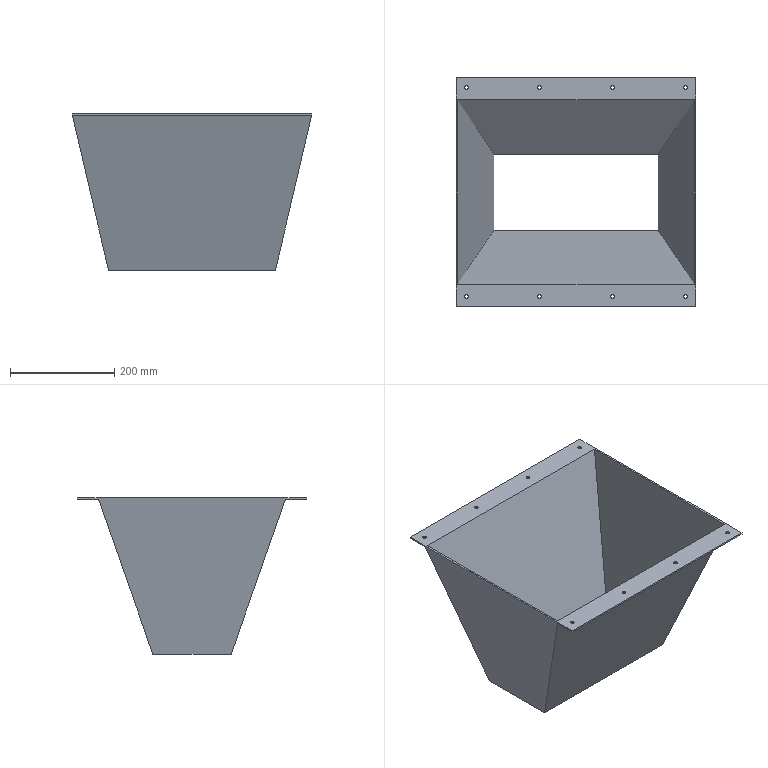Part | SolidWorks | features ICE 7, Extrusion 1, HoleWzd 1, LPattern 1, MirrorPattern 1, Shell 1 | 1 solid | 42 faces | box 460 x 440 x 300 mm | volume 1312965 mm3 | plane 26 | cylinder 16 | commonest cylinder face diameters 7 x16
STEP:
#1=CARTESIAN_POINT('',(206.5,-200.,-3.));
#2=VERTEX_POINT('',#1);
#3=CARTESIAN_POINT('',(213.5,-200.,-3.));
#4=VERTEX_POINT('',#3);
#5=CARTESIAN_POINT('',(210.,-200.,-3.));
#6=DIRECTION('',(0.,0.,1.));
#7=DIRECTION('',(1.,0.,0.));
#8=AXIS2_PLACEMENT_3D('',#5,#6,#7);
#9=CIRCLE('',#8,3.5);
#10=EDGE_CURVE('',#2,#4,#9,.T.);
#11=ORIENTED_EDGE('',*,*,#10,.F.);
#12=CARTESIAN_POINT('',(206.5,-200.,0.));
#13=VERTEX_POINT('',#12);
#14=CARTESIAN_POINT('',(206.5,-200.,0.));
#15=DIRECTION('',(0.,0.,1.));
#16=VECTOR('',#15,1000.);
#17=LINE('',#14,#16);
#18=EDGE_CURVE('',#2,#13,#17,.T.);
#19=ORIENTED_EDGE('',*,*,#18,.T.);
#20=CARTESIAN_POINT('',(213.5,-200.,0.));
#21=VERTEX_POINT('',#20);
#22=CARTESIAN_POINT('',(210.,-200.,0.));
#23=DIRECTION('',(0.,0.,1.));
#24=DIRECTION('',(1.,0.,0.));
#25=AXIS2_PLACEMENT_3D('',#22,#23,#24);
#26=CIRCLE('',#25,3.5);
#27=EDGE_CURVE('',#13,#21,#26,.T.);
#28=ORIENTED_EDGE('',*,*,#27,.T.);
#29=CARTESIAN_POINT('',(213.5,-200.,0.));
#30=DIRECTION('',(0.,0.,1.));
#31=VECTOR('',#30,1000.);
#32=LINE('',#29,#31);
#33=EDGE_CURVE('',#4,#21,#32,.T.);
#34=ORIENTED_EDGE('',*,*,#33,.F.);
#35=EDGE_LOOP('',(#11,#19,#28,#34));
#36=FACE_OUTER_BOUND('',#35,.T.);
#37=CARTESIAN_POINT('',(210.,-200.,0.));
#38=DIRECTION('',(0.,0.,1.));
#39=DIRECTION('',(1.,0.,0.));
#40=AXIS2_PLACEMENT_3D('',#37,#38,#39);
#41=CYLINDRICAL_SURFACE('',#40,3.5);
#42=ADVANCED_FACE('',(#36),#41,.F.);
#43=CARTESIAN_POINT('',(66.5,-200.,-3.));
#44=VERTEX_POINT('',#43);
#45=CARTESIAN_POINT('',(73.5,-200.,-3.));
#46=VERTEX_POINT('',#45);
#47=CARTESIAN_POINT('',(70.,-200.,-3.));
#48=DIRECTION('',(0.,0.,1.));
#49=DIRECTION('',(1.,0.,0.));
#50=AXIS2_PLACEMENT_3D('',#47,#48,#49);
#51=CIRCLE('',#50,3.5);
#52=EDGE_CURVE('',#44,#46,#51,.T.);
#53=ORIENTED_EDGE('',*,*,#52,.F.);
#54=CARTESIAN_POINT('',(66.5,-200.,0.));
#55=VERTEX_POINT('',#54);
#56=CARTESIAN_POINT('',(66.5,-200.,0.));
#57=DIRECTION('',(0.,0.,1.));
#58=VECTOR('',#57,1000.);
#59=LINE('',#56,#58);
#60=EDGE_CURVE('',#44,#55,#59,.T.);
#61=ORIENTED_EDGE('',*,*,#60,.T.);
#62=CARTESIAN_POINT('',(73.5,-200.,0.));
#63=VERTEX_POINT('',#62);
#64=CARTESIAN_POINT('',(70.,-200.,0.));
#65=DIRECTION('',(0.,0.,1.));
#66=DIRECTION('',(1.,0.,0.));
#67=AXIS2_PLACEMENT_3D('',#64,#65,#66);
#68=CIRCLE('',#67,3.5);
#69=EDGE_CURVE('',#55,#63,#68,.T.);
#70=ORIENTED_EDGE('',*,*,#69,.T.);
#71=CARTESIAN_POINT('',(73.5,-200.,0.));
#72=DIRECTION('',(0.,0.,1.));
#73=VECTOR('',#72,1000.);
#74=LINE('',#71,#73);
#75=EDGE_CURVE('',#46,#63,#74,.T.);
#76=ORIENTED_EDGE('',*,*,#75,.F.);
#77=EDGE_LOOP('',(#53,#61,#70,#76));
#78=FACE_OUTER_BOUND('',#77,.T.);
#79=CARTESIAN_POINT('',(70.,-200.,0.));
#80=DIRECTION('',(0.,0.,1.));
#81=DIRECTION('',(1.,0.,0.));
#82=AXIS2_PLACEMENT_3D('',#79,#80,#81);
#83=CYLINDRICAL_SURFACE('',#82,3.5);
#84=ADVANCED_FACE('',(#78),#83,.F.);
#85=CARTESIAN_POINT('',(-73.5,-200.,-3.));
#86=VERTEX_POINT('',#85);
#87=CARTESIAN_POINT('',(-66.5,-200.,-3.));
#88=VERTEX_POINT('',#87);
#89=CARTESIAN_POINT('',(-70.,-200.,-3.));
#90=DIRECTION('',(0.,0.,1.));
#91=DIRECTION('',(1.,0.,0.));
#92=AXIS2_PLACEMENT_3D('',#89,#90,#91);
#93=CIRCLE('',#92,3.5);
#94=EDGE_CURVE('',#86,#88,#93,.T.);
#95=ORIENTED_EDGE('',*,*,#94,.F.);
#96=CARTESIAN_POINT('',(-73.5,-200.,0.));
#97=VERTEX_POINT('',#96);
#98=CARTESIAN_POINT('',(-73.5,-200.,0.));
#99=DIRECTION('',(0.,0.,1.));
#100=VECTOR('',#99,1000.);
#101=LINE('',#98,#100);
#102=EDGE_CURVE('',#86,#97,#101,.T.);
#103=ORIENTED_EDGE('',*,*,#102,.T.);
#104=CARTESIAN_POINT('',(-66.5,-200.,0.));
#105=VERTEX_POINT('',#104);
#106=CARTESIAN_POINT('',(-70.,-200.,0.));
#107=DIRECTION('',(0.,0.,1.));
#108=DIRECTION('',(1.,0.,0.));
#109=AXIS2_PLACEMENT_3D('',#106,#107,#108);
#110=CIRCLE('',#109,3.5);
#111=EDGE_CURVE('',#97,#105,#110,.T.);
#112=ORIENTED_EDGE('',*,*,#111,.T.);
#113=CARTESIAN_POINT('',(-66.5,-200.,0.));
#114=DIRECTION('',(0.,0.,1.));
#115=VECTOR('',#114,1000.);
#116=LINE('',#113,#115);
#117=EDGE_CURVE('',#88,#105,#116,.T.);
#118=ORIENTED_EDGE('',*,*,#117,.F.);
#119=EDGE_LOOP('',(#95,#103,#112,#118));
#120=FACE_OUTER_BOUND('',#119,.T.);
#121=CARTESIAN_POINT('',(-70.,-200.,0.));
#122=DIRECTION('',(0.,0.,1.));
#123=DIRECTION('',(1.,0.,0.));
#124=AXIS2_PLACEMENT_3D('',#121,#122,#123);
#125=CYLINDRICAL_SURFACE('',#124,3.5);
#126=ADVANCED_FACE('',(#120),#125,.F.);
#127=CARTESIAN_POINT('',(-213.5,-200.,-3.));
#128=VERTEX_POINT('',#127);
#129=CARTESIAN_POINT('',(-206.5,-200.,-3.));
#130=VERTEX_POINT('',#129);
#131=CARTESIAN_POINT('',(-210.,-200.,-3.));
#132=DIRECTION('',(0.,0.,1.));
#133=DIRECTION('',(1.,0.,0.));
#134=AXIS2_PLACEMENT_3D('',#131,#132,#133);
#135=CIRCLE('',#134,3.5);
#136=EDGE_CURVE('',#128,#130,#135,.T.);
#137=ORIENTED_EDGE('',*,*,#136,.F.);
#138=CARTESIAN_POINT('',(-213.5,-200.,0.));
#139=VERTEX_POINT('',#138);
#140=CARTESIAN_POINT('',(-213.5,-200.,0.));
#141=DIRECTION('',(0.,0.,1.));
#142=VECTOR('',#141,1000.);
#143=LINE('',#140,#142);
#144=EDGE_CURVE('',#128,#139,#143,.T.);
#145=ORIENTED_EDGE('',*,*,#144,.T.);
#146=CARTESIAN_POINT('',(-206.5,-200.,0.));
#147=VERTEX_POINT('',#146);
#148=CARTESIAN_POINT('',(-210.,-200.,0.));
#149=DIRECTION('',(0.,0.,1.));
#150=DIRECTION('',(1.,0.,0.));
#151=AXIS2_PLACEMENT_3D('',#148,#149,#150);
#152=CIRCLE('',#151,3.5);
#153=EDGE_CURVE('',#139,#147,#152,.T.);
#154=ORIENTED_EDGE('',*,*,#153,.T.);
#155=CARTESIAN_POINT('',(-206.5,-200.,0.));
#156=DIRECTION('',(0.,0.,1.));
#157=VECTOR('',#156,1000.);
#158=LINE('',#155,#157);
#159=EDGE_CURVE('',#130,#147,#158,.T.);
#160=ORIENTED_EDGE('',*,*,#159,.F.);
#161=EDGE_LOOP('',(#137,#145,#154,#160));
#162=FACE_OUTER_BOUND('',#161,.T.);
#163=CARTESIAN_POINT('',(-210.,-200.,0.));
#164=DIRECTION('',(0.,0.,1.));
#165=DIRECTION('',(1.,0.,0.));
#166=AXIS2_PLACEMENT_3D('',#163,#164,#165);
#167=CYLINDRICAL_SURFACE('',#166,3.5);
#168=ADVANCED_FACE('',(#162),#167,.F.);
#169=CARTESIAN_POINT('',(206.5,200.,-3.));
#170=VERTEX_POINT('',#169);
#171=CARTESIAN_POINT('',(213.5,200.,-3.));
#172=VERTEX_POINT('',#171);
#173=CARTESIAN_POINT('',(210.,200.,-3.));
#174=DIRECTION('',(0.,0.,1.));
#175=DIRECTION('',(1.,0.,0.));
#176=AXIS2_PLACEMENT_3D('',#173,#174,#175);
#177=CIRCLE('',#176,3.5);
#178=EDGE_CURVE('',#170,#172,#177,.T.);
#179=ORIENTED_EDGE('',*,*,#178,.F.);
#180=CARTESIAN_POINT('',(206.5,200.,0.));
#181=VERTEX_POINT('',#180);
#182=CARTESIAN_POINT('',(206.5,200.,0.));
#183=DIRECTION('',(0.,0.,1.));
#184=VECTOR('',#183,1000.);
#185=LINE('',#182,#184);
#186=EDGE_CURVE('',#170,#181,#185,.T.);
#187=ORIENTED_EDGE('',*,*,#186,.T.);
#188=CARTESIAN_POINT('',(213.5,200.,0.));
#189=VERTEX_POINT('',#188);
#190=CARTESIAN_POINT('',(210.,200.,0.));
#191=DIRECTION('',(0.,0.,1.));
#192=DIRECTION('',(1.,0.,0.));
#193=AXIS2_PLACEMENT_3D('',#190,#191,#192);
#194=CIRCLE('',#193,3.5);
#195=EDGE_CURVE('',#181,#189,#194,.T.);
#196=ORIENTED_EDGE('',*,*,#195,.T.);
#197=CARTESIAN_POINT('',(213.5,200.,0.));
#198=DIRECTION('',(0.,0.,1.));
#199=VECTOR('',#198,1000.);
#200=LINE('',#197,#199);
#201=EDGE_CURVE('',#172,#189,#200,.T.);
#202=ORIENTED_EDGE('',*,*,#201,.F.);
#203=EDGE_LOOP('',(#179,#187,#196,#202));
#204=FACE_OUTER_BOUND('',#203,.T.);
#205=CARTESIAN_POINT('',(210.,200.,0.));
#206=DIRECTION('',(0.,0.,1.));
#207=DIRECTION('',(1.,0.,0.));
#208=AXIS2_PLACEMENT_3D('',#205,#206,#207);
#209=CYLINDRICAL_SURFACE('',#208,3.5);
#210=ADVANCED_FACE('',(#204),#209,.F.);
#211=CARTESIAN_POINT('',(66.5,200.,-3.));
#212=VERTEX_POINT('',#211);
#213=CARTESIAN_POINT('',(73.5,200.,-3.));
#214=VERTEX_POINT('',#213);
#215=CARTESIAN_POINT('',(70.,200.,-3.));
#216=DIRECTION('',(0.,0.,1.));
#217=DIRECTION('',(1.,0.,0.));
#218=AXIS2_PLACEMENT_3D('',#215,#216,#217);
#219=CIRCLE('',#218,3.5);
#220=EDGE_CURVE('',#212,#214,#219,.T.);
#221=ORIENTED_EDGE('',*,*,#220,.F.);
#222=CARTESIAN_POINT('',(66.5,200.,0.));
#223=VERTEX_POINT('',#222);
#224=CARTESIAN_POINT('',(66.5,200.,0.));
#225=DIRECTION('',(0.,0.,1.));
#226=VECTOR('',#225,1000.);
#227=LINE('',#224,#226);
#228=EDGE_CURVE('',#212,#223,#227,.T.);
#229=ORIENTED_EDGE('',*,*,#228,.T.);
#230=CARTESIAN_POINT('',(73.5,200.,0.));
#231=VERTEX_POINT('',#230);
#232=CARTESIAN_POINT('',(70.,200.,0.));
#233=DIRECTION('',(0.,0.,1.));
#234=DIRECTION('',(1.,0.,0.));
#235=AXIS2_PLACEMENT_3D('',#232,#233,#234);
#236=CIRCLE('',#235,3.5);
#237=EDGE_CURVE('',#223,#231,#236,.T.);
#238=ORIENTED_EDGE('',*,*,#237,.T.);
#239=CARTESIAN_POINT('',(73.5,200.,0.));
#240=DIRECTION('',(0.,0.,1.));
#241=VECTOR('',#240,1000.);
#242=LINE('',#239,#241);
#243=EDGE_CURVE('',#214,#231,#242,.T.);
#244=ORIENTED_EDGE('',*,*,#243,.F.);
#245=EDGE_LOOP('',(#221,#229,#238,#244));
#246=FACE_OUTER_BOUND('',#245,.T.);
#247=CARTESIAN_POINT('',(70.,200.,0.));
#248=DIRECTION('',(0.,0.,1.));
#249=DIRECTION('',(1.,0.,0.));
#250=AXIS2_PLACEMENT_3D('',#247,#248,#249);
#251=CYLINDRICAL_SURFACE('',#250,3.5);
#252=ADVANCED_FACE('',(#246),#251,.F.);
#253=CARTESIAN_POINT('',(-73.5,200.,-3.));
#254=VERTEX_POINT('',#253);
#255=CARTESIAN_POINT('',(-66.5,200.,-3.));
#256=VERTEX_POINT('',#255);
#257=CARTESIAN_POINT('',(-70.,200.,-3.));
#258=DIRECTION('',(0.,0.,1.));
#259=DIRECTION('',(1.,0.,0.));
#260=AXIS2_PLACEMENT_3D('',#257,#258,#259);
#261=CIRCLE('',#260,3.5);
#262=EDGE_CURVE('',#254,#256,#261,.T.);
#263=ORIENTED_EDGE('',*,*,#262,.F.);
#264=CARTESIAN_POINT('',(-73.5,200.,0.));
#265=VERTEX_POINT('',#264);
#266=CARTESIAN_POINT('',(-73.5,200.,0.));
#267=DIRECTION('',(0.,0.,1.));
#268=VECTOR('',#267,1000.);
#269=LINE('',#266,#268);
#270=EDGE_CURVE('',#254,#265,#269,.T.);
#271=ORIENTED_EDGE('',*,*,#270,.T.);
#272=CARTESIAN_POINT('',(-66.5,200.,0.));
#273=VERTEX_POINT('',#272);
#274=CARTESIAN_POINT('',(-70.,200.,0.));
#275=DIRECTION('',(0.,0.,1.));
#276=DIRECTION('',(1.,0.,0.));
#277=AXIS2_PLACEMENT_3D('',#274,#275,#276);
#278=CIRCLE('',#277,3.5);
#279=EDGE_CURVE('',#265,#273,#278,.T.);
#280=ORIENTED_EDGE('',*,*,#279,.T.);
#281=CARTESIAN_POINT('',(-66.5,200.,0.));
#282=DIRECTION('',(0.,0.,1.));
#283=VECTOR('',#282,1000.);
#284=LINE('',#281,#283);
#285=EDGE_CURVE('',#256,#273,#284,.T.);
#286=ORIENTED_EDGE('',*,*,#285,.F.);
#287=EDGE_LOOP('',(#263,#271,#280,#286));
#288=FACE_OUTER_BOUND('',#287,.T.);
#289=CARTESIAN_POINT('',(-70.,200.,0.));
#290=DIRECTION('',(0.,0.,1.));
#291=DIRECTION('',(1.,0.,0.));
#292=AXIS2_PLACEMENT_3D('',#289,#290,#291);
#293=CYLINDRICAL_SURFACE('',#292,3.5);
#294=ADVANCED_FACE('',(#288),#293,.F.);
#295=CARTESIAN_POINT('',(-213.5,200.,-3.));
#296=VERTEX_POINT('',#295);
#297=CARTESIAN_POINT('',(-206.5,200.,-3.));
#298=VERTEX_POINT('',#297);
#299=CARTESIAN_POINT('',(-210.,200.,-3.));
#300=DIRECTION('',(0.,0.,1.));
#301=DIRECTION('',(1.,0.,0.));
#302=AXIS2_PLACEMENT_3D('',#299,#300,#301);
#303=CIRCLE('',#302,3.5);
#304=EDGE_CURVE('',#296,#298,#303,.T.);
#305=ORIENTED_EDGE('',*,*,#304,.F.);
#306=CARTESIAN_POINT('',(-213.5,200.,0.));
#307=VERTEX_POINT('',#306);
#308=CARTESIAN_POINT('',(-213.5,200.,0.));
#309=DIRECTION('',(0.,0.,1.));
#310=VECTOR('',#309,1000.);
#311=LINE('',#308,#310);
#312=EDGE_CURVE('',#296,#307,#311,.T.);
#313=ORIENTED_EDGE('',*,*,#312,.T.);
#314=CARTESIAN_POINT('',(-206.5,200.,0.));
#315=VERTEX_POINT('',#314);
#316=CARTESIAN_POINT('',(-210.,200.,0.));
#317=DIRECTION('',(0.,0.,1.));
#318=DIRECTION('',(1.,0.,0.));
#319=AXIS2_PLACEMENT_3D('',#316,#317,#318);
#320=CIRCLE('',#319,3.5);
#321=EDGE_CURVE('',#307,#315,#320,.T.);
#322=ORIENTED_EDGE('',*,*,#321,.T.);
#323=CARTESIAN_POINT('',(-206.5,200.,0.));
#324=DIRECTION('',(0.,0.,1.));
#325=VECTOR('',#324,1000.);
#326=LINE('',#323,#325);
#327=EDGE_CURVE('',#298,#315,#326,.T.);
#328=ORIENTED_EDGE('',*,*,#327,.F.);
#329=EDGE_LOOP('',(#305,#313,#322,#328));
#330=FACE_OUTER_BOUND('',#329,.T.);
#331=CARTESIAN_POINT('',(-210.,200.,0.));
#332=DIRECTION('',(0.,0.,1.));
#333=DIRECTION('',(1.,0.,0.));
#334=AXIS2_PLACEMENT_3D('',#331,#332,#333);
#335=CYLINDRICAL_SURFACE('',#334,3.5);
#336=ADVANCED_FACE('',(#330),#335,.F.);
#337=CARTESIAN_POINT('',(-157.619,-72.872,-300.));
#338=VERTEX_POINT('',#337);
#339=CARTESIAN_POINT('',(157.619,-72.872,-300.));
#340=VERTEX_POINT('',#339);
#341=CARTESIAN_POINT('',(-157.619,-72.872,-300.));
#342=DIRECTION('',(1.,0.,0.));
#343=VECTOR('',#342,1000.);
#344=LINE('',#341,#343);
#345=EDGE_CURVE('',#338,#340,#344,.T.);
#346=ORIENTED_EDGE('',*,*,#345,.T.);
#347=CARTESIAN_POINT('',(157.619,72.872,-300.));
#348=VERTEX_POINT('',#347);
#349=CARTESIAN_POINT('',(157.619,-72.872,-300.));
#350=DIRECTION('',(0.,1.,0.));
#351=VECTOR('',#350,1000.);
#352=LINE('',#349,#351);
#353=EDGE_CURVE('',#340,#348,#352,.T.);
#354=ORIENTED_EDGE('',*,*,#353,.T.);
#355=CARTESIAN_POINT('',(-157.619,72.872,-300.));
#356=VERTEX_POINT('',#355);
#357=CARTESIAN_POINT('',(157.619,72.872,-300.));
#358=DIRECTION('',(-1.,0.,0.));
#359=VECTOR('',#358,1000.);
#360=LINE('',#357,#359);
#361=EDGE_CURVE('',#348,#356,#360,.T.);
#362=ORIENTED_EDGE('',*,*,#361,.T.);
#363=CARTESIAN_POINT('',(-157.619,72.872,-300.));
#364=DIRECTION('',(0.,-1.,0.));
#365=VECTOR('',#364,1000.);
#366=LINE('',#363,#365);
#367=EDGE_CURVE('',#356,#338,#366,.T.);
#368=ORIENTED_EDGE('',*,*,#367,.T.);
#369=EDGE_LOOP('',(#346,#354,#362,#368));
#370=FACE_BOUND('',#369,.T.);
#371=CARTESIAN_POINT('',(-160.,75.,-300.));
#372=VERTEX_POINT('',#371);
#373=CARTESIAN_POINT('',(160.,75.,-300.));
#374=VERTEX_POINT('',#373);
#375=CARTESIAN_POINT('',(-230.,75.,-300.));
#376=DIRECTION('',(1.,0.,0.));
#377=VECTOR('',#376,1000.);
#378=LINE('',#375,#377);
#379=EDGE_CURVE('',#372,#374,#378,.T.);
#380=ORIENTED_EDGE('',*,*,#379,.T.);
#381=CARTESIAN_POINT('',(160.,-75.,-300.));
#382=VERTEX_POINT('',#381);
#383=CARTESIAN_POINT('',(160.,-302.,-300.));
#384=DIRECTION('',(0.,1.,0.));
#385=VECTOR('',#384,1000.);
#386=LINE('',#383,#385);
#387=EDGE_CURVE('',#382,#374,#386,.T.);
#388=ORIENTED_EDGE('',*,*,#387,.F.);
#389=CARTESIAN_POINT('',(-160.,-75.,-300.));
#390=VERTEX_POINT('',#389);
#391=CARTESIAN_POINT('',(-230.,-75.,-300.));
#392=DIRECTION('',(1.,0.,0.));
#393=VECTOR('',#392,1000.);
#394=LINE('',#391,#393);
#395=EDGE_CURVE('',#390,#382,#394,.T.);
#396=ORIENTED_EDGE('',*,*,#395,.F.);
#397=CARTESIAN_POINT('',(-160.,-302.,-300.));
#398=DIRECTION('',(0.,1.,0.));
#399=VECTOR('',#398,1000.);
#400=LINE('',#397,#399);
#401=EDGE_CURVE('',#390,#372,#400,.T.);
#402=ORIENTED_EDGE('',*,*,#401,.T.);
#403=EDGE_LOOP('',(#380,#388,#396,#402));
#404=FACE_OUTER_BOUND('',#403,.T.);
#405=CARTESIAN_POINT('',(0.,0.,-300.));
#406=DIRECTION('',(0.,0.,1.));
#407=DIRECTION('',(1.,0.,0.));
#408=AXIS2_PLACEMENT_3D('',#405,#406,#407);
#409=PLANE('',#408);
#410=ADVANCED_FACE('',(#370,#404),#409,.F.);
#411=CARTESIAN_POINT('',(210.,-200.,0.));
#412=DIRECTION('',(0.,0.,1.));
#413=DIRECTION('',(1.,0.,0.));
#414=AXIS2_PLACEMENT_3D('',#411,#412,#413);
#415=CIRCLE('',#414,3.5);
#416=EDGE_CURVE('',#21,#13,#415,.T.);
#417=ORIENTED_EDGE('',*,*,#416,.F.);
#418=ORIENTED_EDGE('',*,*,#27,.F.);
#419=EDGE_LOOP('',(#417,#418));
#420=FACE_BOUND('',#419,.T.);
#421=CARTESIAN_POINT('',(70.,-200.,0.));
#422=DIRECTION('',(0.,0.,1.));
#423=DIRECTION('',(1.,0.,0.));
#424=AXIS2_PLACEMENT_3D('',#421,#422,#423);
#425=CIRCLE('',#424,3.5);
#426=EDGE_CURVE('',#63,#55,#425,.T.);
#427=ORIENTED_EDGE('',*,*,#426,.F.);
#428=ORIENTED_EDGE('',*,*,#69,.F.);
#429=EDGE_LOOP('',(#427,#428));
#430=FACE_BOUND('',#429,.T.);
#431=CARTESIAN_POINT('',(-70.,-200.,0.));
#432=DIRECTION('',(0.,0.,1.));
#433=DIRECTION('',(1.,0.,0.));
#434=AXIS2_PLACEMENT_3D('',#431,#432,#433);
#435=CIRCLE('',#434,3.5);
#436=EDGE_CURVE('',#105,#97,#435,.T.);
#437=ORIENTED_EDGE('',*,*,#436,.F.);
#438=ORIENTED_EDGE('',*,*,#111,.F.);
#439=EDGE_LOOP('',(#437,#438));
#440=FACE_BOUND('',#439,.T.);
#441=CARTESIAN_POINT('',(-210.,-200.,0.));
#442=DIRECTION('',(0.,0.,1.));
#443=DIRECTION('',(1.,0.,0.));
#444=AXIS2_PLACEMENT_3D('',#441,#442,#443);
#445=CIRCLE('',#444,3.5);
#446=EDGE_CURVE('',#147,#139,#445,.T.);
#447=ORIENTED_EDGE('',*,*,#446,.F.);
#448=ORIENTED_EDGE('',*,*,#153,.F.);
#449=EDGE_LOOP('',(#447,#448));
#450=FACE_BOUND('',#449,.T.);
#451=CARTESIAN_POINT('',(-70.,200.,0.));
#452=DIRECTION('',(0.,0.,1.));
#453=DIRECTION('',(1.,0.,0.));
#454=AXIS2_PLACEMENT_3D('',#451,#452,#453);
#455=CIRCLE('',#454,3.5);
#456=EDGE_CURVE('',#273,#265,#455,.T.);
#457=ORIENTED_EDGE('',*,*,#456,.F.);
#458=ORIENTED_EDGE('',*,*,#279,.F.);
#459=EDGE_LOOP('',(#457,#458));
#460=FACE_BOUND('',#459,.T.);
#461=CARTESIAN_POINT('',(-210.,200.,0.));
#462=DIRECTION('',(0.,0.,1.));
#463=DIRECTION('',(1.,0.,0.));
#464=AXIS2_PLACEMENT_3D('',#461,#462,#463);
#465=CIRCLE('',#464,3.5);
#466=EDGE_CURVE('',#315,#307,#465,.T.);
#467=ORIENTED_EDGE('',*,*,#466,.F.);
#468=ORIENTED_EDGE('',*,*,#321,.F.);
#469=EDGE_LOOP('',(#467,#468));
#470=FACE_BOUND('',#469,.T.);
#471=CARTESIAN_POINT('',(226.919,-176.822,0.));
#472=VERTEX_POINT('',#471);
#473=CARTESIAN_POINT('',(226.919,176.822,0.));
#474=VERTEX_POINT('',#473);
#475=CARTESIAN_POINT('',(226.919,-302.,0.));
#476=DIRECTION('',(0.,1.,0.));
#477=VECTOR('',#476,1000.);
#478=LINE('',#475,#477);
#479=EDGE_CURVE('',#472,#474,#478,.T.);
#480=ORIENTED_EDGE('',*,*,#479,.F.);
#481=CARTESIAN_POINT('',(-226.919,-176.822,0.));
#482=VERTEX_POINT('',#481);
#483=CARTESIAN_POINT('',(-230.,-176.822,0.));
#484=DIRECTION('',(1.,0.,0.));
#485=VECTOR('',#484,1000.);
#486=LINE('',#483,#485);
#487=EDGE_CURVE('',#482,#472,#486,.T.);
#488=ORIENTED_EDGE('',*,*,#487,.F.);
#489=CARTESIAN_POINT('',(-226.919,176.822,0.));
#490=VERTEX_POINT('',#489);
#491=CARTESIAN_POINT('',(-226.919,-302.,0.));
#492=DIRECTION('',(0.,-1.,0.));
#493=VECTOR('',#492,1000.);
#494=LINE('',#491,#493);
#495=EDGE_CURVE('',#490,#482,#494,.T.);
#496=ORIENTED_EDGE('',*,*,#495,.F.);
#497=CARTESIAN_POINT('',(-230.,176.822,0.));
#498=DIRECTION('',(-1.,0.,0.));
#499=VECTOR('',#498,1000.);
#500=LINE('',#497,#499);
#501=EDGE_CURVE('',#474,#490,#500,.T.);
#502=ORIENTED_EDGE('',*,*,#501,.F.);
#503=EDGE_LOOP('',(#480,#488,#496,#502));
#504=FACE_BOUND('',#503,.T.);
#505=CARTESIAN_POINT('',(230.,-180.,0.));
#506=VERTEX_POINT('',#505);
#507=CARTESIAN_POINT('',(230.,180.,0.));
#508=VERTEX_POINT('',#507);
#509=CARTESIAN_POINT('',(230.,180.,0.));
#510=DIRECTION('',(0.,1.,0.));
#511=VECTOR('',#510,1000.);
#512=LINE('',#509,#511);
#513=EDGE_CURVE('',#506,#508,#512,.T.);
#514=ORIENTED_EDGE('',*,*,#513,.T.);
#515=CARTESIAN_POINT('',(230.,220.,0.));
#516=VERTEX_POINT('',#515);
#517=CARTESIAN_POINT('',(230.,180.,0.));
#518=DIRECTION('',(0.,1.,0.));
#519=VECTOR('',#518,1000.);
#520=LINE('',#517,#519);
#521=EDGE_CURVE('',#508,#516,#520,.T.);
#522=ORIENTED_EDGE('',*,*,#521,.T.);
#523=CARTESIAN_POINT('',(-230.,220.,0.));
#524=VERTEX_POINT('',#523);
#525=CARTESIAN_POINT('',(-230.,220.,0.));
#526=DIRECTION('',(-1.,0.,0.));
#527=VECTOR('',#526,1000.);
#528=LINE('',#525,#527);
#529=EDGE_CURVE('',#516,#524,#528,.T.);
#530=ORIENTED_EDGE('',*,*,#529,.T.);
#531=CARTESIAN_POINT('',(-230.,180.,0.));
#532=VERTEX_POINT('',#531);
#533=CARTESIAN_POINT('',(-230.,180.,0.));
#534=DIRECTION('',(0.,-1.,0.));
#535=VECTOR('',#534,1000.);
#536=LINE('',#533,#535);
#537=EDGE_CURVE('',#524,#532,#536,.T.);
#538=ORIENTED_EDGE('',*,*,#537,.T.);
#539=CARTESIAN_POINT('',(-230.,-180.,0.));
#540=VERTEX_POINT('',#539);
#541=CARTESIAN_POINT('',(-230.,180.,0.));
#542=DIRECTION('',(0.,-1.,0.));
#543=VECTOR('',#542,1000.);
#544=LINE('',#541,#543);
#545=EDGE_CURVE('',#532,#540,#544,.T.);
#546=ORIENTED_EDGE('',*,*,#545,.T.);
#547=CARTESIAN_POINT('',(-230.,-220.,0.));
#548=VERTEX_POINT('',#547);
#549=CARTESIAN_POINT('',(-230.,-180.,0.));
#550=DIRECTION('',(0.,-1.,0.));
#551=VECTOR('',#550,1000.);
#552=LINE('',#549,#551);
#553=EDGE_CURVE('',#540,#548,#552,.T.);
#554=ORIENTED_EDGE('',*,*,#553,.T.);
#555=CARTESIAN_POINT('',(230.,-220.,0.));
#556=VERTEX_POINT('',#555);
#557=CARTESIAN_POINT('',(-230.,-220.,0.));
#558=DIRECTION('',(1.,0.,0.));
#559=VECTOR('',#558,1000.);
#560=LINE('',#557,#559);
#561=EDGE_CURVE('',#548,#556,#560,.T.);
#562=ORIENTED_EDGE('',*,*,#561,.T.);
#563=CARTESIAN_POINT('',(230.,-180.,0.));
#564=DIRECTION('',(0.,1.,0.));
#565=VECTOR('',#564,1000.);
#566=LINE('',#563,#565);
#567=EDGE_CURVE('',#556,#506,#566,.T.);
#568=ORIENTED_EDGE('',*,*,#567,.T.);
#569=EDGE_LOOP('',(#514,#522,#530,#538,#546,#554,#562,#568));
#570=FACE_OUTER_BOUND('',#569,.T.);
#571=CARTESIAN_POINT('',(70.,200.,0.));
#572=DIRECTION('',(0.,0.,1.));
#573=DIRECTION('',(1.,0.,0.));
#574=AXIS2_PLACEMENT_3D('',#571,#572,#573);
#575=CIRCLE('',#574,3.5);
#576=EDGE_CURVE('',#231,#223,#575,.T.);
#577=ORIENTED_EDGE('',*,*,#576,.F.);
#578=ORIENTED_EDGE('',*,*,#237,.F.);
#579=EDGE_LOOP('',(#577,#578));
#580=FACE_BOUND('',#579,.T.);
#581=CARTESIAN_POINT('',(210.,200.,0.));
#582=DIRECTION('',(0.,0.,1.));
#583=DIRECTION('',(1.,0.,0.));
#584=AXIS2_PLACEMENT_3D('',#581,#582,#583);
#585=CIRCLE('',#584,3.5);
#586=EDGE_CURVE('',#189,#181,#585,.T.);
#587=ORIENTED_EDGE('',*,*,#586,.F.);
#588=ORIENTED_EDGE('',*,*,#195,.F.);
#589=EDGE_LOOP('',(#587,#588));
#590=FACE_BOUND('',#589,.T.);
#591=CARTESIAN_POINT('',(0.,0.,0.));
#592=DIRECTION('',(0.,0.,1.));
#593=DIRECTION('',(1.,0.,0.));
#594=AXIS2_PLACEMENT_3D('',#591,#592,#593);
#595=PLANE('',#594);
#596=ADVANCED_FACE('',(#420,#430,#440,#450,#460,#470,#504,#570,#580,#590),#595,.T.);
#597=CARTESIAN_POINT('',(-229.3,178.95,-3.));
#598=VERTEX_POINT('',#597);
#599=CARTESIAN_POINT('',(-230.,180.,0.));
#600=DIRECTION('',(-0.2151,0.3226,0.9218));
#601=VECTOR('',#600,1000.);
#602=LINE('',#599,#601);
#603=EDGE_CURVE('',#372,#598,#602,.T.);
#604=ORIENTED_EDGE('',*,*,#603,.T.);
#605=CARTESIAN_POINT('',(229.3,178.95,-3.));
#606=VERTEX_POINT('',#605);
#607=CARTESIAN_POINT('',(-230.,178.95,-3.));
#608=DIRECTION('',(1.,0.,0.));
#609=VECTOR('',#608,1000.);
#610=LINE('',#607,#609);
#611=EDGE_CURVE('',#598,#606,#610,.T.);
#612=ORIENTED_EDGE('',*,*,#611,.T.);
#613=CARTESIAN_POINT('',(208.721,148.081,-91.197));
#614=DIRECTION('',(-0.2151,-0.3226,-0.9218));
#615=VECTOR('',#614,1000.);
#616=LINE('',#613,#615);
#617=EDGE_CURVE('',#606,#374,#616,.T.);
#618=ORIENTED_EDGE('',*,*,#617,.T.);
#619=ORIENTED_EDGE('',*,*,#379,.F.);
#620=EDGE_LOOP('',(#604,#612,#618,#619));
#621=FACE_OUTER_BOUND('',#620,.T.);
#622=CARTESIAN_POINT('',(-230.,180.,0.));
#623=DIRECTION('',(0.,-0.9439,0.3304));
#624=DIRECTION('',(0.,-0.3304,-0.9439));
#625=AXIS2_PLACEMENT_3D('',#622,#623,#624);
#626=PLANE('',#625);
#627=ADVANCED_FACE('',(#621),#626,.F.);
#628=CARTESIAN_POINT('',(229.3,-178.95,-3.));
#629=VERTEX_POINT('',#628);
#630=CARTESIAN_POINT('',(208.721,-148.081,-91.197));
#631=DIRECTION('',(0.2151,-0.3226,0.9218));
#632=VECTOR('',#631,1000.);
#633=LINE('',#630,#632);
#634=EDGE_CURVE('',#382,#629,#633,.T.);
#635=ORIENTED_EDGE('',*,*,#634,.T.);
#636=CARTESIAN_POINT('',(-229.3,-178.95,-3.));
#637=VERTEX_POINT('',#636);
#638=CARTESIAN_POINT('',(230.,-178.95,-3.));
#639=DIRECTION('',(-1.,0.,0.));
#640=VECTOR('',#639,1000.);
#641=LINE('',#638,#640);
#642=EDGE_CURVE('',#629,#637,#641,.T.);
#643=ORIENTED_EDGE('',*,*,#642,.T.);
#644=CARTESIAN_POINT('',(-230.,-180.,0.));
#645=DIRECTION('',(0.2151,0.3226,-0.9218));
#646=VECTOR('',#645,1000.);
#647=LINE('',#644,#646);
#648=EDGE_CURVE('',#637,#390,#647,.T.);
#649=ORIENTED_EDGE('',*,*,#648,.T.);
#650=ORIENTED_EDGE('',*,*,#395,.T.);
#651=EDGE_LOOP('',(#635,#643,#649,#650));
#652=FACE_OUTER_BOUND('',#651,.T.);
#653=CARTESIAN_POINT('',(-230.,-180.,0.));
#654=DIRECTION('',(0.,0.9439,0.3304));
#655=DIRECTION('',(0.,-0.3304,0.9439));
#656=AXIS2_PLACEMENT_3D('',#653,#654,#655);
#657=PLANE('',#656);
#658=ADVANCED_FACE('',(#652),#657,.F.);
#659=ORIENTED_EDGE('',*,*,#401,.F.);
#660=ORIENTED_EDGE('',*,*,#648,.F.);
#661=CARTESIAN_POINT('',(-230.,-180.,0.));
#662=DIRECTION('',(0.2151,0.3226,-0.9218));
#663=VECTOR('',#662,1000.);
#664=LINE('',#661,#663);
#665=EDGE_CURVE('',#540,#637,#664,.T.);
#666=ORIENTED_EDGE('',*,*,#665,.F.);
#667=ORIENTED_EDGE('',*,*,#545,.F.);
#668=CARTESIAN_POINT('',(-230.,180.,0.));
#669=DIRECTION('',(-0.2151,0.3226,0.9218));
#670=VECTOR('',#669,1000.);
#671=LINE('',#668,#670);
#672=EDGE_CURVE('',#598,#532,#671,.T.);
#673=ORIENTED_EDGE('',*,*,#672,.F.);
#674=ORIENTED_EDGE('',*,*,#603,.F.);
#675=EDGE_LOOP('',(#659,#660,#666,#667,#673,#674));
#676=FACE_OUTER_BOUND('',#675,.T.);
#677=CARTESIAN_POINT('',(-230.,-302.,0.));
#678=DIRECTION('',(0.9738,0.,0.2272));
#679=DIRECTION('',(0.2272,0.,-0.9738));
#680=AXIS2_PLACEMENT_3D('',#677,#678,#679);
#681=PLANE('',#680);
#682=ADVANCED_FACE('',(#676),#681,.F.);
#683=ORIENTED_EDGE('',*,*,#513,.F.);
#684=CARTESIAN_POINT('',(208.721,-148.081,-91.197));
#685=DIRECTION('',(0.2151,-0.3226,0.9218));
#686=VECTOR('',#685,1000.);
#687=LINE('',#684,#686);
#688=EDGE_CURVE('',#629,#506,#687,.T.);
#689=ORIENTED_EDGE('',*,*,#688,.F.);
#690=ORIENTED_EDGE('',*,*,#634,.F.);
#691=ORIENTED_EDGE('',*,*,#387,.T.);
#692=ORIENTED_EDGE('',*,*,#617,.F.);
#693=CARTESIAN_POINT('',(208.721,148.081,-91.197));
#694=DIRECTION('',(-0.2151,-0.3226,-0.9218));
#695=VECTOR('',#694,1000.);
#696=LINE('',#693,#695);
#697=EDGE_CURVE('',#508,#606,#696,.T.);
#698=ORIENTED_EDGE('',*,*,#697,.F.);
#699=EDGE_LOOP('',(#683,#689,#690,#691,#692,#698));
#700=FACE_OUTER_BOUND('',#699,.T.);
#701=CARTESIAN_POINT('',(230.,-302.,0.));
#702=DIRECTION('',(-0.9738,0.,0.2272));
#703=DIRECTION('',(0.2272,0.,0.9738));
#704=AXIS2_PLACEMENT_3D('',#701,#702,#703);
#705=PLANE('',#704);
#706=ADVANCED_FACE('',(#700),#705,.F.);
#707=ORIENTED_EDGE('',*,*,#501,.T.);
#708=CARTESIAN_POINT('',(-157.619,72.872,-297.));
#709=VERTEX_POINT('',#708);
#710=CARTESIAN_POINT('',(-227.282,177.366,1.556));
#711=DIRECTION('',(-0.2151,0.3226,0.9218));
#712=VECTOR('',#711,1000.);
#713=LINE('',#710,#712);
#714=EDGE_CURVE('',#709,#490,#713,.T.);
#715=ORIENTED_EDGE('',*,*,#714,.F.);
#716=CARTESIAN_POINT('',(157.619,72.872,-297.));
#717=VERTEX_POINT('',#716);
#718=CARTESIAN_POINT('',(0.,72.872,-297.));
#719=DIRECTION('',(1.,0.,0.));
#720=VECTOR('',#719,1000.);
#721=LINE('',#718,#720);
#722=EDGE_CURVE('',#709,#717,#721,.T.);
#723=ORIENTED_EDGE('',*,*,#722,.T.);
#724=CARTESIAN_POINT('',(206.003,145.447,-89.641));
#725=DIRECTION('',(-0.2151,-0.3226,-0.9218));
#726=VECTOR('',#725,1000.);
#727=LINE('',#724,#726);
#728=EDGE_CURVE('',#474,#717,#727,.T.);
#729=ORIENTED_EDGE('',*,*,#728,.F.);
#730=EDGE_LOOP('',(#707,#715,#723,#729));
#731=FACE_OUTER_BOUND('',#730,.T.);
#732=CARTESIAN_POINT('',(-230.,177.168,0.9911));
#733=DIRECTION('',(0.,-0.9439,0.3304));
#734=DIRECTION('',(0.,-0.3304,-0.9439));
#735=AXIS2_PLACEMENT_3D('',#732,#733,#734);
#736=PLANE('',#735);
#737=ADVANCED_FACE('',(#731),#736,.T.);
#738=CARTESIAN_POINT('',(-157.619,-72.872,-297.));
#739=VERTEX_POINT('',#738);
#740=CARTESIAN_POINT('',(157.619,-72.872,-297.));
#741=VERTEX_POINT('',#740);
#742=CARTESIAN_POINT('',(-230.,-72.872,-297.));
#743=DIRECTION('',(1.,0.,0.));
#744=VECTOR('',#743,1000.);
#745=LINE('',#742,#744);
#746=EDGE_CURVE('',#739,#741,#745,.T.);
#747=ORIENTED_EDGE('',*,*,#746,.F.);
#748=CARTESIAN_POINT('',(-227.282,-177.366,1.556));
#749=DIRECTION('',(0.2151,0.3226,-0.9218));
#750=VECTOR('',#749,1000.);
#751=LINE('',#748,#750);
#752=EDGE_CURVE('',#482,#739,#751,.T.);
#753=ORIENTED_EDGE('',*,*,#752,.F.);
#754=ORIENTED_EDGE('',*,*,#487,.T.);
#755=CARTESIAN_POINT('',(206.003,-145.447,-89.641));
#756=DIRECTION('',(0.2151,-0.3226,0.9218));
#757=VECTOR('',#756,1000.);
#758=LINE('',#755,#757);
#759=EDGE_CURVE('',#741,#472,#758,.T.);
#760=ORIENTED_EDGE('',*,*,#759,.F.);
#761=EDGE_LOOP('',(#747,#753,#754,#760));
#762=FACE_OUTER_BOUND('',#761,.T.);
#763=CARTESIAN_POINT('',(-230.,-177.168,0.9911));
#764=DIRECTION('',(0.,0.9439,0.3304));
#765=DIRECTION('',(0.,-0.3304,0.9439));
#766=AXIS2_PLACEMENT_3D('',#763,#764,#765);
#767=PLANE('',#766);
#768=ADVANCED_FACE('',(#762),#767,.T.);
#769=CARTESIAN_POINT('',(-157.619,0.,-297.));
#770=DIRECTION('',(0.,1.,0.));
#771=VECTOR('',#770,1000.);
#772=LINE('',#769,#771);
#773=EDGE_CURVE('',#739,#709,#772,.T.);
#774=ORIENTED_EDGE('',*,*,#773,.T.);
#775=ORIENTED_EDGE('',*,*,#714,.T.);
#776=ORIENTED_EDGE('',*,*,#495,.T.);
#777=ORIENTED_EDGE('',*,*,#752,.T.);
#778=EDGE_LOOP('',(#774,#775,#776,#777));
#779=FACE_OUTER_BOUND('',#778,.T.);
#780=CARTESIAN_POINT('',(-227.078,-302.,0.6817));
#781=DIRECTION('',(0.9738,0.,0.2272));
#782=DIRECTION('',(0.2272,0.,-0.9738));
#783=AXIS2_PLACEMENT_3D('',#780,#781,#782);
#784=PLANE('',#783);
#785=ADVANCED_FACE('',(#779),#784,.T.);
#786=ORIENTED_EDGE('',*,*,#479,.T.);
#787=ORIENTED_EDGE('',*,*,#728,.T.);
#788=CARTESIAN_POINT('',(157.619,-302.,-297.));
#789=DIRECTION('',(0.,1.,0.));
#790=VECTOR('',#789,1000.);
#791=LINE('',#788,#790);
#792=EDGE_CURVE('',#741,#717,#791,.T.);
#793=ORIENTED_EDGE('',*,*,#792,.F.);
#794=ORIENTED_EDGE('',*,*,#759,.T.);
#795=EDGE_LOOP('',(#786,#787,#793,#794));
#796=FACE_OUTER_BOUND('',#795,.T.);
#797=CARTESIAN_POINT('',(227.078,-302.,0.6817));
#798=DIRECTION('',(-0.9738,0.,0.2272));
#799=DIRECTION('',(0.2272,0.,0.9738));
#800=AXIS2_PLACEMENT_3D('',#797,#798,#799);
#801=PLANE('',#800);
#802=ADVANCED_FACE('',(#796),#801,.T.);
#803=ORIENTED_EDGE('',*,*,#792,.T.);
#804=CARTESIAN_POINT('',(157.619,72.872,-300.));
#805=DIRECTION('',(0.,0.,1.));
#806=VECTOR('',#805,1000.);
#807=LINE('',#804,#806);
#808=EDGE_CURVE('',#348,#717,#807,.T.);
#809=ORIENTED_EDGE('',*,*,#808,.F.);
#810=ORIENTED_EDGE('',*,*,#353,.F.);
#811=CARTESIAN_POINT('',(157.619,-72.872,-300.));
#812=DIRECTION('',(0.,0.,1.));
#813=VECTOR('',#812,1000.);
#814=LINE('',#811,#813);
#815=EDGE_CURVE('',#340,#741,#814,.T.);
#816=ORIENTED_EDGE('',*,*,#815,.T.);
#817=EDGE_LOOP('',(#803,#809,#810,#816));
#818=FACE_OUTER_BOUND('',#817,.T.);
#819=CARTESIAN_POINT('',(157.619,-72.872,-300.));
#820=DIRECTION('',(1.,0.,0.));
#821=DIRECTION('',(0.,0.,-1.));
#822=AXIS2_PLACEMENT_3D('',#819,#820,#821);
#823=PLANE('',#822);
#824=ADVANCED_FACE('',(#818),#823,.F.);
#825=ORIENTED_EDGE('',*,*,#746,.T.);
#826=ORIENTED_EDGE('',*,*,#815,.F.);
#827=ORIENTED_EDGE('',*,*,#345,.F.);
#828=CARTESIAN_POINT('',(-157.619,-72.872,-300.));
#829=DIRECTION('',(0.,0.,1.));
#830=VECTOR('',#829,1000.);
#831=LINE('',#828,#830);
#832=EDGE_CURVE('',#338,#739,#831,.T.);
#833=ORIENTED_EDGE('',*,*,#832,.T.);
#834=EDGE_LOOP('',(#825,#826,#827,#833));
#835=FACE_OUTER_BOUND('',#834,.T.);
#836=CARTESIAN_POINT('',(-157.619,-72.872,-300.));
#837=DIRECTION('',(0.,-1.,0.));
#838=DIRECTION('',(0.,0.,-1.));
#839=AXIS2_PLACEMENT_3D('',#836,#837,#838);
#840=PLANE('',#839);
#841=ADVANCED_FACE('',(#835),#840,.F.);
#842=ORIENTED_EDGE('',*,*,#773,.F.);
#843=ORIENTED_EDGE('',*,*,#832,.F.);
#844=ORIENTED_EDGE('',*,*,#367,.F.);
#845=CARTESIAN_POINT('',(-157.619,72.872,-300.));
#846=DIRECTION('',(0.,0.,1.));
#847=VECTOR('',#846,1000.);
#848=LINE('',#845,#847);
#849=EDGE_CURVE('',#356,#709,#848,.T.);
#850=ORIENTED_EDGE('',*,*,#849,.T.);
#851=EDGE_LOOP('',(#842,#843,#844,#850));
#852=FACE_OUTER_BOUND('',#851,.T.);
#853=CARTESIAN_POINT('',(-157.619,72.872,-300.));
#854=DIRECTION('',(-1.,0.,0.));
#855=DIRECTION('',(0.,0.,1.));
#856=AXIS2_PLACEMENT_3D('',#853,#854,#855);
#857=PLANE('',#856);
#858=ADVANCED_FACE('',(#852),#857,.F.);
#859=ORIENTED_EDGE('',*,*,#722,.F.);
#860=ORIENTED_EDGE('',*,*,#849,.F.);
#861=ORIENTED_EDGE('',*,*,#361,.F.);
#862=ORIENTED_EDGE('',*,*,#808,.T.);
#863=EDGE_LOOP('',(#859,#860,#861,#862));
#864=FACE_OUTER_BOUND('',#863,.T.);
#865=CARTESIAN_POINT('',(157.619,72.872,-300.));
#866=DIRECTION('',(0.,1.,0.));
#867=DIRECTION('',(0.,0.,1.));
#868=AXIS2_PLACEMENT_3D('',#865,#866,#867);
#869=PLANE('',#868);
#870=ADVANCED_FACE('',(#864),#869,.F.);
#871=CARTESIAN_POINT('',(230.,-178.95,-3.));
#872=VERTEX_POINT('',#871);
#873=CARTESIAN_POINT('',(230.,-178.95,-3.));
#874=DIRECTION('',(-1.,0.,0.));
#875=VECTOR('',#874,1000.);
#876=LINE('',#873,#875);
#877=EDGE_CURVE('',#872,#629,#876,.T.);
#878=ORIENTED_EDGE('',*,*,#877,.T.);
#879=ORIENTED_EDGE('',*,*,#688,.T.);
#880=CARTESIAN_POINT('',(230.,-128.248,-147.862));
#881=DIRECTION('',(0.,0.3304,-0.9439));
#882=VECTOR('',#881,1000.);
#883=LINE('',#880,#882);
#884=EDGE_CURVE('',#506,#872,#883,.T.);
#885=ORIENTED_EDGE('',*,*,#884,.T.);
#886=EDGE_LOOP('',(#878,#879,#885));
#887=FACE_OUTER_BOUND('',#886,.T.);
#888=CARTESIAN_POINT('',(-230.,-180.,0.));
#889=DIRECTION('',(0.,0.9439,0.3304));
#890=DIRECTION('',(0.,-0.3304,0.9439));
#891=AXIS2_PLACEMENT_3D('',#888,#889,#890);
#892=PLANE('',#891);
#893=ADVANCED_FACE('',(#887),#892,.T.);
#894=CARTESIAN_POINT('',(-230.,-178.95,-3.));
#895=VERTEX_POINT('',#894);
#896=CARTESIAN_POINT('',(-230.,-127.313,-150.535));
#897=DIRECTION('',(0.,-0.3304,0.9439));
#898=VECTOR('',#897,1000.);
#899=LINE('',#896,#898);
#900=EDGE_CURVE('',#895,#540,#899,.T.);
#901=ORIENTED_EDGE('',*,*,#900,.T.);
#902=ORIENTED_EDGE('',*,*,#665,.T.);
#903=CARTESIAN_POINT('',(230.,-178.95,-3.));
#904=DIRECTION('',(-1.,0.,0.));
#905=VECTOR('',#904,1000.);
#906=LINE('',#903,#905);
#907=EDGE_CURVE('',#637,#895,#906,.T.);
#908=ORIENTED_EDGE('',*,*,#907,.T.);
#909=EDGE_LOOP('',(#901,#902,#908));
#910=FACE_OUTER_BOUND('',#909,.T.);
#911=CARTESIAN_POINT('',(-230.,-180.,0.));
#912=DIRECTION('',(0.,0.9439,0.3304));
#913=DIRECTION('',(0.,-0.3304,0.9439));
#914=AXIS2_PLACEMENT_3D('',#911,#912,#913);
#915=PLANE('',#914);
#916=ADVANCED_FACE('',(#910),#915,.T.);
#917=CARTESIAN_POINT('',(210.,-200.,-3.));
#918=DIRECTION('',(0.,0.,1.));
#919=DIRECTION('',(1.,0.,0.));
#920=AXIS2_PLACEMENT_3D('',#917,#918,#919);
#921=CIRCLE('',#920,3.5);
#922=EDGE_CURVE('',#4,#2,#921,.T.);
#923=ORIENTED_EDGE('',*,*,#922,.T.);
#924=ORIENTED_EDGE('',*,*,#10,.T.);
#925=EDGE_LOOP('',(#923,#924));
#926=FACE_BOUND('',#925,.T.);
#927=CARTESIAN_POINT('',(70.,-200.,-3.));
#928=DIRECTION('',(0.,0.,1.));
#929=DIRECTION('',(1.,0.,0.));
#930=AXIS2_PLACEMENT_3D('',#927,#928,#929);
#931=CIRCLE('',#930,3.5);
#932=EDGE_CURVE('',#46,#44,#931,.T.);
#933=ORIENTED_EDGE('',*,*,#932,.T.);
#934=ORIENTED_EDGE('',*,*,#52,.T.);
#935=EDGE_LOOP('',(#933,#934));
#936=FACE_BOUND('',#935,.T.);
#937=CARTESIAN_POINT('',(-70.,-200.,-3.));
#938=DIRECTION('',(0.,0.,1.));
#939=DIRECTION('',(1.,0.,0.));
#940=AXIS2_PLACEMENT_3D('',#937,#938,#939);
#941=CIRCLE('',#940,3.5);
#942=EDGE_CURVE('',#88,#86,#941,.T.);
#943=ORIENTED_EDGE('',*,*,#942,.T.);
#944=ORIENTED_EDGE('',*,*,#94,.T.);
#945=EDGE_LOOP('',(#943,#944));
#946=FACE_BOUND('',#945,.T.);
#947=CARTESIAN_POINT('',(-210.,-200.,-3.));
#948=DIRECTION('',(0.,0.,1.));
#949=DIRECTION('',(1.,0.,0.));
#950=AXIS2_PLACEMENT_3D('',#947,#948,#949);
#951=CIRCLE('',#950,3.5);
#952=EDGE_CURVE('',#130,#128,#951,.T.);
#953=ORIENTED_EDGE('',*,*,#952,.T.);
#954=ORIENTED_EDGE('',*,*,#136,.T.);
#955=EDGE_LOOP('',(#953,#954));
#956=FACE_BOUND('',#955,.T.);
#957=ORIENTED_EDGE('',*,*,#877,.F.);
#958=CARTESIAN_POINT('',(230.,-220.,-3.));
#959=VERTEX_POINT('',#958);
#960=CARTESIAN_POINT('',(230.,294.216,-3.));
#961=DIRECTION('',(0.,-1.,0.));
#962=VECTOR('',#961,1000.);
#963=LINE('',#960,#962);
#964=EDGE_CURVE('',#872,#959,#963,.T.);
#965=ORIENTED_EDGE('',*,*,#964,.T.);
#966=CARTESIAN_POINT('',(-230.,-220.,-3.));
#967=VERTEX_POINT('',#966);
#968=CARTESIAN_POINT('',(-230.,-220.,-3.));
#969=DIRECTION('',(1.,0.,0.));
#970=VECTOR('',#969,1000.);
#971=LINE('',#968,#970);
#972=EDGE_CURVE('',#967,#959,#971,.T.);
#973=ORIENTED_EDGE('',*,*,#972,.F.);
#974=CARTESIAN_POINT('',(-230.,294.216,-3.));
#975=DIRECTION('',(0.,-1.,0.));
#976=VECTOR('',#975,1000.);
#977=LINE('',#974,#976);
#978=EDGE_CURVE('',#895,#967,#977,.T.);
#979=ORIENTED_EDGE('',*,*,#978,.F.);
#980=ORIENTED_EDGE('',*,*,#907,.F.);
#981=ORIENTED_EDGE('',*,*,#642,.F.);
#982=EDGE_LOOP('',(#957,#965,#973,#979,#980,#981));
#983=FACE_OUTER_BOUND('',#982,.T.);
#984=CARTESIAN_POINT('',(230.,294.216,-3.));
#985=DIRECTION('',(0.,0.,1.));
#986=DIRECTION('',(1.,0.,0.));
#987=AXIS2_PLACEMENT_3D('',#984,#985,#986);
#988=PLANE('',#987);
#989=ADVANCED_FACE('',(#926,#936,#946,#956,#983),#988,.F.);
#990=ORIENTED_EDGE('',*,*,#884,.F.);
#991=ORIENTED_EDGE('',*,*,#567,.F.);
#992=CARTESIAN_POINT('',(230.,-220.,-3.));
#993=DIRECTION('',(0.,0.,1.));
#994=VECTOR('',#993,1000.);
#995=LINE('',#992,#994);
#996=EDGE_CURVE('',#959,#556,#995,.T.);
#997=ORIENTED_EDGE('',*,*,#996,.F.);
#998=ORIENTED_EDGE('',*,*,#964,.F.);
#999=EDGE_LOOP('',(#990,#991,#997,#998));
#1000=FACE_OUTER_BOUND('',#999,.T.);
#1001=CARTESIAN_POINT('',(230.,294.216,0.));
#1002=DIRECTION('',(-1.,0.,0.));
#1003=DIRECTION('',(0.,-1.,0.));
#1004=AXIS2_PLACEMENT_3D('',#1001,#1002,#1003);
#1005=PLANE('',#1004);
#1006=ADVANCED_FACE('',(#1000),#1005,.F.);
#1007=ORIENTED_EDGE('',*,*,#900,.F.);
#1008=ORIENTED_EDGE('',*,*,#978,.T.);
#1009=CARTESIAN_POINT('',(-230.,-220.,-3.));
#1010=DIRECTION('',(0.,0.,1.));
#1011=VECTOR('',#1010,1000.);
#1012=LINE('',#1009,#1011);
#1013=EDGE_CURVE('',#967,#548,#1012,.T.);
#1014=ORIENTED_EDGE('',*,*,#1013,.T.);
#1015=ORIENTED_EDGE('',*,*,#553,.F.);
#1016=EDGE_LOOP('',(#1007,#1008,#1014,#1015));
#1017=FACE_OUTER_BOUND('',#1016,.T.);
#1018=CARTESIAN_POINT('',(-230.,294.216,-3.));
#1019=DIRECTION('',(1.,0.,0.));
#1020=DIRECTION('',(0.,1.,0.));
#1021=AXIS2_PLACEMENT_3D('',#1018,#1019,#1020);
#1022=PLANE('',#1021);
#1023=ADVANCED_FACE('',(#1017),#1022,.F.);
#1024=ORIENTED_EDGE('',*,*,#561,.F.);
#1025=ORIENTED_EDGE('',*,*,#1013,.F.);
#1026=ORIENTED_EDGE('',*,*,#972,.T.);
#1027=ORIENTED_EDGE('',*,*,#996,.T.);
#1028=EDGE_LOOP('',(#1024,#1025,#1026,#1027));
#1029=FACE_OUTER_BOUND('',#1028,.T.);
#1030=CARTESIAN_POINT('',(-230.,-220.,-3.));
#1031=DIRECTION('',(0.,-1.,0.));
#1032=DIRECTION('',(1.,0.,0.));
#1033=AXIS2_PLACEMENT_3D('',#1030,#1031,#1032);
#1034=PLANE('',#1033);
#1035=ADVANCED_FACE('',(#1029),#1034,.T.);
#1036=CARTESIAN_POINT('',(230.,178.95,-3.));
#1037=VERTEX_POINT('',#1036);
#1038=CARTESIAN_POINT('',(230.,127.313,-150.535));
#1039=DIRECTION('',(0.,0.3304,0.9439));
#1040=VECTOR('',#1039,1000.);
#1041=LINE('',#1038,#1040);
#1042=EDGE_CURVE('',#1037,#508,#1041,.T.);
#1043=ORIENTED_EDGE('',*,*,#1042,.T.);
#1044=ORIENTED_EDGE('',*,*,#697,.T.);
#1045=CARTESIAN_POINT('',(-230.,178.95,-3.));
#1046=DIRECTION('',(1.,0.,0.));
#1047=VECTOR('',#1046,1000.);
#1048=LINE('',#1045,#1047);
#1049=EDGE_CURVE('',#606,#1037,#1048,.T.);
#1050=ORIENTED_EDGE('',*,*,#1049,.T.);
#1051=EDGE_LOOP('',(#1043,#1044,#1050));
#1052=FACE_OUTER_BOUND('',#1051,.T.);
#1053=CARTESIAN_POINT('',(-230.,180.,0.));
#1054=DIRECTION('',(0.,-0.9439,0.3304));
#1055=DIRECTION('',(0.,-0.3304,-0.9439));
#1056=AXIS2_PLACEMENT_3D('',#1053,#1054,#1055);
#1057=PLANE('',#1056);
#1058=ADVANCED_FACE('',(#1052),#1057,.T.);
#1059=CARTESIAN_POINT('',(-230.,178.95,-3.));
#1060=VERTEX_POINT('',#1059);
#1061=CARTESIAN_POINT('',(-230.,178.95,-3.));
#1062=DIRECTION('',(1.,0.,0.));
#1063=VECTOR('',#1062,1000.);
#1064=LINE('',#1061,#1063);
#1065=EDGE_CURVE('',#1060,#598,#1064,.T.);
#1066=ORIENTED_EDGE('',*,*,#1065,.T.);
#1067=ORIENTED_EDGE('',*,*,#672,.T.);
#1068=CARTESIAN_POINT('',(-230.,128.248,-147.862));
#1069=DIRECTION('',(0.,-0.3304,-0.9439));
#1070=VECTOR('',#1069,1000.);
#1071=LINE('',#1068,#1070);
#1072=EDGE_CURVE('',#532,#1060,#1071,.T.);
#1073=ORIENTED_EDGE('',*,*,#1072,.T.);
#1074=EDGE_LOOP('',(#1066,#1067,#1073));
#1075=FACE_OUTER_BOUND('',#1074,.T.);
#1076=CARTESIAN_POINT('',(-230.,180.,0.));
#1077=DIRECTION('',(0.,-0.9439,0.3304));
#1078=DIRECTION('',(0.,-0.3304,-0.9439));
#1079=AXIS2_PLACEMENT_3D('',#1076,#1077,#1078);
#1080=PLANE('',#1079);
#1081=ADVANCED_FACE('',(#1075),#1080,.T.);
#1082=CARTESIAN_POINT('',(-70.,200.,-3.));
#1083=DIRECTION('',(0.,0.,1.));
#1084=DIRECTION('',(1.,0.,0.));
#1085=AXIS2_PLACEMENT_3D('',#1082,#1083,#1084);
#1086=CIRCLE('',#1085,3.5);
#1087=EDGE_CURVE('',#256,#254,#1086,.T.);
#1088=ORIENTED_EDGE('',*,*,#1087,.T.);
#1089=ORIENTED_EDGE('',*,*,#262,.T.);
#1090=EDGE_LOOP('',(#1088,#1089));
#1091=FACE_BOUND('',#1090,.T.);
#1092=CARTESIAN_POINT('',(-210.,200.,-3.));
#1093=DIRECTION('',(0.,0.,1.));
#1094=DIRECTION('',(1.,0.,0.));
#1095=AXIS2_PLACEMENT_3D('',#1092,#1093,#1094);
#1096=CIRCLE('',#1095,3.5);
#1097=EDGE_CURVE('',#298,#296,#1096,.T.);
#1098=ORIENTED_EDGE('',*,*,#1097,.T.);
#1099=ORIENTED_EDGE('',*,*,#304,.T.);
#1100=EDGE_LOOP('',(#1098,#1099));
#1101=FACE_BOUND('',#1100,.T.);
#1102=ORIENTED_EDGE('',*,*,#1065,.F.);
#1103=CARTESIAN_POINT('',(-230.,220.,-3.));
#1104=VERTEX_POINT('',#1103);
#1105=CARTESIAN_POINT('',(-230.,-294.216,-3.));
#1106=DIRECTION('',(0.,1.,0.));
#1107=VECTOR('',#1106,1000.);
#1108=LINE('',#1105,#1107);
#1109=EDGE_CURVE('',#1060,#1104,#1108,.T.);
#1110=ORIENTED_EDGE('',*,*,#1109,.T.);
#1111=CARTESIAN_POINT('',(230.,220.,-3.));
#1112=VERTEX_POINT('',#1111);
#1113=CARTESIAN_POINT('',(-230.,220.,-3.));
#1114=DIRECTION('',(-1.,0.,0.));
#1115=VECTOR('',#1114,1000.);
#1116=LINE('',#1113,#1115);
#1117=EDGE_CURVE('',#1112,#1104,#1116,.T.);
#1118=ORIENTED_EDGE('',*,*,#1117,.F.);
#1119=CARTESIAN_POINT('',(230.,-294.216,-3.));
#1120=DIRECTION('',(0.,1.,0.));
#1121=VECTOR('',#1120,1000.);
#1122=LINE('',#1119,#1121);
#1123=EDGE_CURVE('',#1037,#1112,#1122,.T.);
#1124=ORIENTED_EDGE('',*,*,#1123,.F.);
#1125=ORIENTED_EDGE('',*,*,#1049,.F.);
#1126=ORIENTED_EDGE('',*,*,#611,.F.);
#1127=EDGE_LOOP('',(#1102,#1110,#1118,#1124,#1125,#1126));
#1128=FACE_OUTER_BOUND('',#1127,.T.);
#1129=CARTESIAN_POINT('',(70.,200.,-3.));
#1130=DIRECTION('',(0.,0.,1.));
#1131=DIRECTION('',(1.,0.,0.));
#1132=AXIS2_PLACEMENT_3D('',#1129,#1130,#1131);
#1133=CIRCLE('',#1132,3.5);
#1134=EDGE_CURVE('',#214,#212,#1133,.T.);
#1135=ORIENTED_EDGE('',*,*,#1134,.T.);
#1136=ORIENTED_EDGE('',*,*,#220,.T.);
#1137=EDGE_LOOP('',(#1135,#1136));
#1138=FACE_BOUND('',#1137,.T.);
#1139=CARTESIAN_POINT('',(210.,200.,-3.));
#1140=DIRECTION('',(0.,0.,1.));
#1141=DIRECTION('',(1.,0.,0.));
#1142=AXIS2_PLACEMENT_3D('',#1139,#1140,#1141);
#1143=CIRCLE('',#1142,3.5);
#1144=EDGE_CURVE('',#172,#170,#1143,.T.);
#1145=ORIENTED_EDGE('',*,*,#1144,.T.);
#1146=ORIENTED_EDGE('',*,*,#178,.T.);
#1147=EDGE_LOOP('',(#1145,#1146));
#1148=FACE_BOUND('',#1147,.T.);
#1149=CARTESIAN_POINT('',(-230.,-294.216,-3.));
#1150=DIRECTION('',(0.,0.,1.));
#1151=DIRECTION('',(1.,0.,0.));
#1152=AXIS2_PLACEMENT_3D('',#1149,#1150,#1151);
#1153=PLANE('',#1152);
#1154=ADVANCED_FACE('',(#1091,#1101,#1128,#1138,#1148),#1153,.F.);
#1155=ORIENTED_EDGE('',*,*,#1072,.F.);
#1156=ORIENTED_EDGE('',*,*,#537,.F.);
#1157=CARTESIAN_POINT('',(-230.,220.,-3.));
#1158=DIRECTION('',(0.,0.,1.));
#1159=VECTOR('',#1158,1000.);
#1160=LINE('',#1157,#1159);
#1161=EDGE_CURVE('',#1104,#524,#1160,.T.);
#1162=ORIENTED_EDGE('',*,*,#1161,.F.);
#1163=ORIENTED_EDGE('',*,*,#1109,.F.);
#1164=EDGE_LOOP('',(#1155,#1156,#1162,#1163));
#1165=FACE_OUTER_BOUND('',#1164,.T.);
#1166=CARTESIAN_POINT('',(-230.,-294.216,0.));
#1167=DIRECTION('',(1.,0.,0.));
#1168=DIRECTION('',(0.,0.,-1.));
#1169=AXIS2_PLACEMENT_3D('',#1166,#1167,#1168);
#1170=PLANE('',#1169);
#1171=ADVANCED_FACE('',(#1165),#1170,.F.);
#1172=ORIENTED_EDGE('',*,*,#1042,.F.);
#1173=ORIENTED_EDGE('',*,*,#1123,.T.);
#1174=CARTESIAN_POINT('',(230.,220.,-3.));
#1175=DIRECTION('',(0.,0.,1.));
#1176=VECTOR('',#1175,1000.);
#1177=LINE('',#1174,#1176);
#1178=EDGE_CURVE('',#1112,#516,#1177,.T.);
#1179=ORIENTED_EDGE('',*,*,#1178,.T.);
#1180=ORIENTED_EDGE('',*,*,#521,.F.);
#1181=EDGE_LOOP('',(#1172,#1173,#1179,#1180));
#1182=FACE_OUTER_BOUND('',#1181,.T.);
#1183=CARTESIAN_POINT('',(230.,-294.216,-3.));
#1184=DIRECTION('',(-1.,0.,0.));
#1185=DIRECTION('',(0.,0.,1.));
#1186=AXIS2_PLACEMENT_3D('',#1183,#1184,#1185);
#1187=PLANE('',#1186);
#1188=ADVANCED_FACE('',(#1182),#1187,.F.);
#1189=ORIENTED_EDGE('',*,*,#529,.F.);
#1190=ORIENTED_EDGE('',*,*,#1178,.F.);
#1191=ORIENTED_EDGE('',*,*,#1117,.T.);
#1192=ORIENTED_EDGE('',*,*,#1161,.T.);
#1193=EDGE_LOOP('',(#1189,#1190,#1191,#1192));
#1194=FACE_OUTER_BOUND('',#1193,.T.);
#1195=CARTESIAN_POINT('',(-230.,220.,-3.));
#1196=DIRECTION('',(0.,1.,0.));
#1197=DIRECTION('',(0.,0.,1.));
#1198=AXIS2_PLACEMENT_3D('',#1195,#1196,#1197);
#1199=PLANE('',#1198);
#1200=ADVANCED_FACE('',(#1194),#1199,.T.);
#1201=ORIENTED_EDGE('',*,*,#312,.F.);
#1202=ORIENTED_EDGE('',*,*,#1097,.F.);
#1203=ORIENTED_EDGE('',*,*,#327,.T.);
#1204=ORIENTED_EDGE('',*,*,#466,.T.);
#1205=EDGE_LOOP('',(#1201,#1202,#1203,#1204));
#1206=FACE_OUTER_BOUND('',#1205,.T.);
#1207=CARTESIAN_POINT('',(-210.,200.,0.));
#1208=DIRECTION('',(0.,0.,1.));
#1209=DIRECTION('',(1.,0.,0.));
#1210=AXIS2_PLACEMENT_3D('',#1207,#1208,#1209);
#1211=CYLINDRICAL_SURFACE('',#1210,3.5);
#1212=ADVANCED_FACE('',(#1206),#1211,.F.);
#1213=ORIENTED_EDGE('',*,*,#270,.F.);
#1214=ORIENTED_EDGE('',*,*,#1087,.F.);
#1215=ORIENTED_EDGE('',*,*,#285,.T.);
#1216=ORIENTED_EDGE('',*,*,#456,.T.);
#1217=EDGE_LOOP('',(#1213,#1214,#1215,#1216));
#1218=FACE_OUTER_BOUND('',#1217,.T.);
#1219=CARTESIAN_POINT('',(-70.,200.,0.));
#1220=DIRECTION('',(0.,0.,1.));
#1221=DIRECTION('',(1.,0.,0.));
#1222=AXIS2_PLACEMENT_3D('',#1219,#1220,#1221);
#1223=CYLINDRICAL_SURFACE('',#1222,3.5);
#1224=ADVANCED_FACE('',(#1218),#1223,.F.);
#1225=ORIENTED_EDGE('',*,*,#228,.F.);
#1226=ORIENTED_EDGE('',*,*,#1134,.F.);
#1227=ORIENTED_EDGE('',*,*,#243,.T.);
#1228=ORIENTED_EDGE('',*,*,#576,.T.);
#1229=EDGE_LOOP('',(#1225,#1226,#1227,#1228));
#1230=FACE_OUTER_BOUND('',#1229,.T.);
#1231=CARTESIAN_POINT('',(70.,200.,0.));
#1232=DIRECTION('',(0.,0.,1.));
#1233=DIRECTION('',(1.,0.,0.));
#1234=AXIS2_PLACEMENT_3D('',#1231,#1232,#1233);
#1235=CYLINDRICAL_SURFACE('',#1234,3.5);
#1236=ADVANCED_FACE('',(#1230),#1235,.F.);
#1237=ORIENTED_EDGE('',*,*,#186,.F.);
#1238=ORIENTED_EDGE('',*,*,#1144,.F.);
#1239=ORIENTED_EDGE('',*,*,#201,.T.);
#1240=ORIENTED_EDGE('',*,*,#586,.T.);
#1241=EDGE_LOOP('',(#1237,#1238,#1239,#1240));
#1242=FACE_OUTER_BOUND('',#1241,.T.);
#1243=CARTESIAN_POINT('',(210.,200.,0.));
#1244=DIRECTION('',(0.,0.,1.));
#1245=DIRECTION('',(1.,0.,0.));
#1246=AXIS2_PLACEMENT_3D('',#1243,#1244,#1245);
#1247=CYLINDRICAL_SURFACE('',#1246,3.5);
#1248=ADVANCED_FACE('',(#1242),#1247,.F.);
#1249=ORIENTED_EDGE('',*,*,#144,.F.);
#1250=ORIENTED_EDGE('',*,*,#952,.F.);
#1251=ORIENTED_EDGE('',*,*,#159,.T.);
#1252=ORIENTED_EDGE('',*,*,#446,.T.);
#1253=EDGE_LOOP('',(#1249,#1250,#1251,#1252));
#1254=FACE_OUTER_BOUND('',#1253,.T.);
#1255=CARTESIAN_POINT('',(-210.,-200.,0.));
#1256=DIRECTION('',(0.,0.,1.));
#1257=DIRECTION('',(1.,0.,0.));
#1258=AXIS2_PLACEMENT_3D('',#1255,#1256,#1257);
#1259=CYLINDRICAL_SURFACE('',#1258,3.5);
#1260=ADVANCED_FACE('',(#1254),#1259,.F.);
#1261=ORIENTED_EDGE('',*,*,#102,.F.);
#1262=ORIENTED_EDGE('',*,*,#942,.F.);
#1263=ORIENTED_EDGE('',*,*,#117,.T.);
#1264=ORIENTED_EDGE('',*,*,#436,.T.);
#1265=EDGE_LOOP('',(#1261,#1262,#1263,#1264));
#1266=FACE_OUTER_BOUND('',#1265,.T.);
#1267=CARTESIAN_POINT('',(-70.,-200.,0.));
#1268=DIRECTION('',(0.,0.,1.));
#1269=DIRECTION('',(1.,0.,0.));
#1270=AXIS2_PLACEMENT_3D('',#1267,#1268,#1269);
#1271=CYLINDRICAL_SURFACE('',#1270,3.5);
#1272=ADVANCED_FACE('',(#1266),#1271,.F.);
#1273=ORIENTED_EDGE('',*,*,#60,.F.);
#1274=ORIENTED_EDGE('',*,*,#932,.F.);
#1275=ORIENTED_EDGE('',*,*,#75,.T.);
#1276=ORIENTED_EDGE('',*,*,#426,.T.);
#1277=EDGE_LOOP('',(#1273,#1274,#1275,#1276));
#1278=FACE_OUTER_BOUND('',#1277,.T.);
#1279=CARTESIAN_POINT('',(70.,-200.,0.));
#1280=DIRECTION('',(0.,0.,1.));
#1281=DIRECTION('',(1.,0.,0.));
#1282=AXIS2_PLACEMENT_3D('',#1279,#1280,#1281);
#1283=CYLINDRICAL_SURFACE('',#1282,3.5);
#1284=ADVANCED_FACE('',(#1278),#1283,.F.);
#1285=ORIENTED_EDGE('',*,*,#18,.F.);
#1286=ORIENTED_EDGE('',*,*,#922,.F.);
#1287=ORIENTED_EDGE('',*,*,#33,.T.);
#1288=ORIENTED_EDGE('',*,*,#416,.T.);
#1289=EDGE_LOOP('',(#1285,#1286,#1287,#1288));
#1290=FACE_OUTER_BOUND('',#1289,.T.);
#1291=CARTESIAN_POINT('',(210.,-200.,0.));
#1292=DIRECTION('',(0.,0.,1.));
#1293=DIRECTION('',(1.,0.,0.));
#1294=AXIS2_PLACEMENT_3D('',#1291,#1292,#1293);
#1295=CYLINDRICAL_SURFACE('',#1294,3.5);
#1296=ADVANCED_FACE('',(#1290),#1295,.F.);
#1297=CLOSED_SHELL('',(#42,#84,#126,#168,#210,#252,#294,#336,#410,#596,#627,#658,#682,#706,#737,#768,#785,#802,#824,#841,#858,#870,#893,#916,#989,#1006,#1023,#1035,#1058,#1081,#1154,#1171,#1188,#1200,#1212,#1224,#1236,#1248,#1260,#1272,#1284,#1296));
#1298=MANIFOLD_SOLID_BREP('',#1297);
#1299=CARTESIAN_POINT('',(0.,0.,0.));
#1300=DIRECTION('',(0.,0.,1.));
#1301=DIRECTION('',(1.,0.,0.));
#1302=AXIS2_PLACEMENT_3D('',#1299,#1300,#1301);
#1303=(LENGTH_UNIT()NAMED_UNIT(*)SI_UNIT(.MILLI.,.METRE.));
#1304=UNCERTAINTY_MEASURE_WITH_UNIT(LENGTH_MEASURE(0.00001),#1303,'','');
#1305=(NAMED_UNIT(*)PLANE_ANGLE_UNIT()SI_UNIT($,.RADIAN.));
#1306=(NAMED_UNIT(*)SI_UNIT($,.STERADIAN.)SOLID_ANGLE_UNIT());
#1307=(GEOMETRIC_REPRESENTATION_CONTEXT(3)GLOBAL_UNCERTAINTY_ASSIGNED_CONTEXT((#1304))GLOBAL_UNIT_ASSIGNED_CONTEXT((#1303,#1305,#1306))REPRESENTATION_CONTEXT('',''));
#1308=ADVANCED_BREP_SHAPE_REPRESENTATION('',(#1298,#1302),#1307);